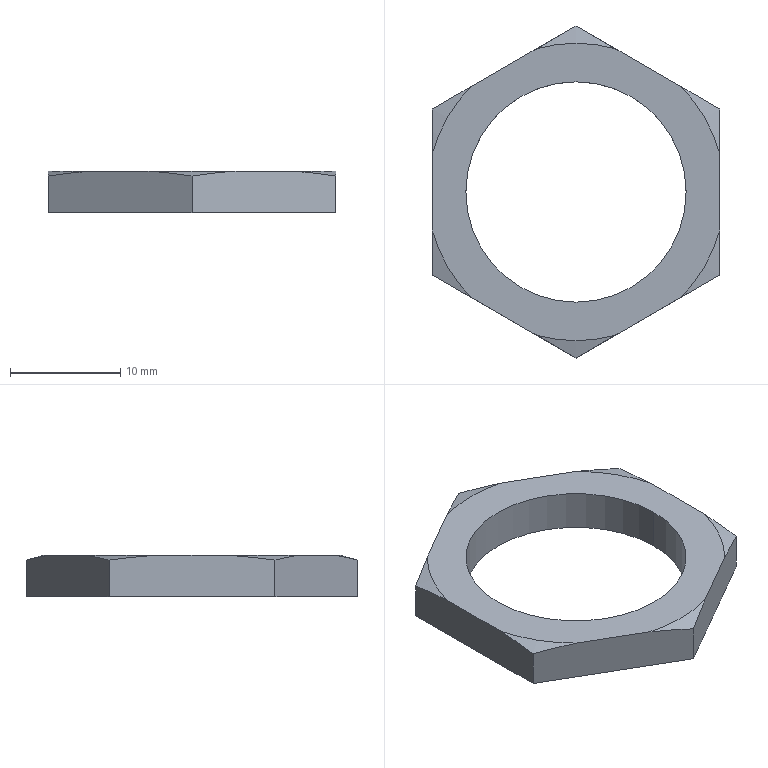Part | STEP file | GB/T 808 M20×1 | 1 solid | 16 faces | box 26.102 x 30.14 x 3.74 mm | volume 1028 mm3 | plane 8 | cone 6 | cylinder 2 | commonest cylinder face diameters 20 x2
STEP:
#1=CARTESIAN_POINT('',(-10.,0.,3.74));
#2=VERTEX_POINT('',#1);
#3=CARTESIAN_POINT('',(10.,0.,3.74));
#4=VERTEX_POINT('',#3);
#5=CARTESIAN_POINT('',(0.,0.,3.74));
#6=DIRECTION('',(0.,0.,1.));
#7=DIRECTION('',(1.,0.,0.));
#8=AXIS2_PLACEMENT_3D('',#5,#6,#7);
#9=CIRCLE('',#8,10.);
#10=EDGE_CURVE('',#2,#4,#9,.T.);
#11=ORIENTED_EDGE('',*,*,#10,.T.);
#12=CARTESIAN_POINT('',(10.,0.,0.));
#13=VERTEX_POINT('',#12);
#14=CARTESIAN_POINT('',(10.,0.,3.74));
#15=DIRECTION('',(0.,0.,-1.));
#16=VECTOR('',#15,1000.);
#17=LINE('',#14,#16);
#18=EDGE_CURVE('',#4,#13,#17,.T.);
#19=ORIENTED_EDGE('',*,*,#18,.T.);
#20=CARTESIAN_POINT('',(-10.,0.,0.));
#21=VERTEX_POINT('',#20);
#22=CARTESIAN_POINT('',(0.,0.,0.));
#23=DIRECTION('',(0.,0.,1.));
#24=DIRECTION('',(1.,0.,0.));
#25=AXIS2_PLACEMENT_3D('',#22,#23,#24);
#26=CIRCLE('',#25,10.);
#27=EDGE_CURVE('',#21,#13,#26,.T.);
#28=ORIENTED_EDGE('',*,*,#27,.F.);
#29=CARTESIAN_POINT('',(-10.,0.,3.74));
#30=DIRECTION('',(0.,0.,-1.));
#31=VECTOR('',#30,1000.);
#32=LINE('',#29,#31);
#33=EDGE_CURVE('',#2,#21,#32,.T.);
#34=ORIENTED_EDGE('',*,*,#33,.F.);
#35=EDGE_LOOP('',(#11,#19,#28,#34));
#36=FACE_OUTER_BOUND('',#35,.T.);
#37=CARTESIAN_POINT('',(0.,0.,3.74));
#38=DIRECTION('',(0.,0.,-1.));
#39=DIRECTION('',(-1.,0.,0.));
#40=AXIS2_PLACEMENT_3D('',#37,#38,#39);
#41=CYLINDRICAL_SURFACE('',#40,10.);
#42=ADVANCED_FACE('',(#36),#41,.F.);
#43=ORIENTED_EDGE('',*,*,#10,.F.);
#44=CARTESIAN_POINT('',(0.,0.,3.74));
#45=DIRECTION('',(0.,0.,1.));
#46=DIRECTION('',(1.,0.,0.));
#47=AXIS2_PLACEMENT_3D('',#44,#45,#46);
#48=CIRCLE('',#47,10.);
#49=EDGE_CURVE('',#4,#2,#48,.T.);
#50=ORIENTED_EDGE('',*,*,#49,.F.);
#51=EDGE_LOOP('',(#43,#50));
#52=FACE_BOUND('',#51,.T.);
#53=CARTESIAN_POINT('',(-9.516,9.576,3.74));
#54=VERTEX_POINT('',#53);
#55=CARTESIAN_POINT('',(-13.051,3.453,3.74));
#56=VERTEX_POINT('',#55);
#57=CARTESIAN_POINT('',(0.,0.,3.74));
#58=DIRECTION('',(0.,0.,1.));
#59=DIRECTION('',(1.,0.,0.));
#60=AXIS2_PLACEMENT_3D('',#57,#58,#59);
#61=CIRCLE('',#60,13.5);
#62=EDGE_CURVE('',#54,#56,#61,.T.);
#63=ORIENTED_EDGE('',*,*,#62,.T.);
#64=CARTESIAN_POINT('',(-13.051,-3.453,3.74));
#65=VERTEX_POINT('',#64);
#66=CARTESIAN_POINT('',(-13.051,7.535,3.74));
#67=DIRECTION('',(0.,-1.,0.));
#68=VECTOR('',#67,1000.);
#69=LINE('',#66,#68);
#70=EDGE_CURVE('',#56,#65,#69,.T.);
#71=ORIENTED_EDGE('',*,*,#70,.T.);
#72=CARTESIAN_POINT('',(-9.516,-9.576,3.74));
#73=VERTEX_POINT('',#72);
#74=CARTESIAN_POINT('',(0.,0.,3.74));
#75=DIRECTION('',(0.,0.,1.));
#76=DIRECTION('',(1.,0.,0.));
#77=AXIS2_PLACEMENT_3D('',#74,#75,#76);
#78=CIRCLE('',#77,13.5);
#79=EDGE_CURVE('',#65,#73,#78,.T.);
#80=ORIENTED_EDGE('',*,*,#79,.T.);
#81=CARTESIAN_POINT('',(-3.535,-13.029,3.74));
#82=VERTEX_POINT('',#81);
#83=CARTESIAN_POINT('',(-13.051,-7.535,3.74));
#84=DIRECTION('',(0.866,-0.5,0.));
#85=VECTOR('',#84,1000.);
#86=LINE('',#83,#85);
#87=EDGE_CURVE('',#73,#82,#86,.T.);
#88=ORIENTED_EDGE('',*,*,#87,.T.);
#89=CARTESIAN_POINT('',(3.535,-13.029,3.74));
#90=VERTEX_POINT('',#89);
#91=CARTESIAN_POINT('',(0.,0.,3.74));
#92=DIRECTION('',(0.,0.,1.));
#93=DIRECTION('',(1.,0.,0.));
#94=AXIS2_PLACEMENT_3D('',#91,#92,#93);
#95=CIRCLE('',#94,13.5);
#96=EDGE_CURVE('',#82,#90,#95,.T.);
#97=ORIENTED_EDGE('',*,*,#96,.T.);
#98=CARTESIAN_POINT('',(9.516,-9.576,3.74));
#99=VERTEX_POINT('',#98);
#100=CARTESIAN_POINT('',(0.,-15.07,3.74));
#101=DIRECTION('',(0.866,0.5,0.));
#102=VECTOR('',#101,1000.);
#103=LINE('',#100,#102);
#104=EDGE_CURVE('',#90,#99,#103,.T.);
#105=ORIENTED_EDGE('',*,*,#104,.T.);
#106=CARTESIAN_POINT('',(13.051,-3.453,3.74));
#107=VERTEX_POINT('',#106);
#108=CARTESIAN_POINT('',(0.,0.,3.74));
#109=DIRECTION('',(0.,0.,1.));
#110=DIRECTION('',(1.,0.,0.));
#111=AXIS2_PLACEMENT_3D('',#108,#109,#110);
#112=CIRCLE('',#111,13.5);
#113=EDGE_CURVE('',#99,#107,#112,.T.);
#114=ORIENTED_EDGE('',*,*,#113,.T.);
#115=CARTESIAN_POINT('',(13.051,3.453,3.74));
#116=VERTEX_POINT('',#115);
#117=CARTESIAN_POINT('',(13.051,-7.535,3.74));
#118=DIRECTION('',(0.,1.,0.));
#119=VECTOR('',#118,1000.);
#120=LINE('',#117,#119);
#121=EDGE_CURVE('',#107,#116,#120,.T.);
#122=ORIENTED_EDGE('',*,*,#121,.T.);
#123=CARTESIAN_POINT('',(9.516,9.576,3.74));
#124=VERTEX_POINT('',#123);
#125=CARTESIAN_POINT('',(0.,0.,3.74));
#126=DIRECTION('',(0.,0.,1.));
#127=DIRECTION('',(1.,0.,0.));
#128=AXIS2_PLACEMENT_3D('',#125,#126,#127);
#129=CIRCLE('',#128,13.5);
#130=EDGE_CURVE('',#116,#124,#129,.T.);
#131=ORIENTED_EDGE('',*,*,#130,.T.);
#132=CARTESIAN_POINT('',(3.535,13.029,3.74));
#133=VERTEX_POINT('',#132);
#134=CARTESIAN_POINT('',(13.051,7.535,3.74));
#135=DIRECTION('',(-0.866,0.5,0.));
#136=VECTOR('',#135,1000.);
#137=LINE('',#134,#136);
#138=EDGE_CURVE('',#124,#133,#137,.T.);
#139=ORIENTED_EDGE('',*,*,#138,.T.);
#140=CARTESIAN_POINT('',(-3.535,13.029,3.74));
#141=VERTEX_POINT('',#140);
#142=CARTESIAN_POINT('',(0.,0.,3.74));
#143=DIRECTION('',(0.,0.,1.));
#144=DIRECTION('',(1.,0.,0.));
#145=AXIS2_PLACEMENT_3D('',#142,#143,#144);
#146=CIRCLE('',#145,13.5);
#147=EDGE_CURVE('',#133,#141,#146,.T.);
#148=ORIENTED_EDGE('',*,*,#147,.T.);
#149=CARTESIAN_POINT('',(0.,15.07,3.74));
#150=DIRECTION('',(-0.866,-0.5,0.));
#151=VECTOR('',#150,1000.);
#152=LINE('',#149,#151);
#153=EDGE_CURVE('',#141,#54,#152,.T.);
#154=ORIENTED_EDGE('',*,*,#153,.T.);
#155=EDGE_LOOP('',(#63,#71,#80,#88,#97,#105,#114,#122,#131,#139,#148,#154));
#156=FACE_OUTER_BOUND('',#155,.T.);
#157=CARTESIAN_POINT('',(26.102,0.,3.74));
#158=DIRECTION('',(0.,0.,-1.));
#159=DIRECTION('',(-1.,0.,0.));
#160=AXIS2_PLACEMENT_3D('',#157,#158,#159);
#161=PLANE('',#160);
#162=ADVANCED_FACE('',(#52,#156),#161,.F.);
#163=CARTESIAN_POINT('',(13.051,7.535,3.319));
#164=VERTEX_POINT('',#163);
#165=CARTESIAN_POINT('',(13.051,7.535,3.319));
#166=CARTESIAN_POINT('',(11.876,8.213,3.501));
#167=CARTESIAN_POINT('',(10.698,8.893,3.646));
#168=CARTESIAN_POINT('',(9.516,9.576,3.74));
#169=B_SPLINE_CURVE_WITH_KNOTS('',3,(#165,#166,#167,#168),.UNSPECIFIED.,.F.,.F.,(4,4),(0.0109,0.01501),.UNSPECIFIED.);
#170=EDGE_CURVE('',#164,#124,#169,.T.);
#171=ORIENTED_EDGE('',*,*,#170,.F.);
#172=CARTESIAN_POINT('',(13.051,7.535,0.));
#173=VERTEX_POINT('',#172);
#174=CARTESIAN_POINT('',(13.051,7.535,3.74));
#175=DIRECTION('',(0.,0.,-1.));
#176=VECTOR('',#175,1000.);
#177=LINE('',#174,#176);
#178=EDGE_CURVE('',#164,#173,#177,.T.);
#179=ORIENTED_EDGE('',*,*,#178,.T.);
#180=CARTESIAN_POINT('',(0.,15.07,0.));
#181=VERTEX_POINT('',#180);
#182=CARTESIAN_POINT('',(13.051,7.535,0.));
#183=DIRECTION('',(-0.866,0.5,0.));
#184=VECTOR('',#183,1000.);
#185=LINE('',#182,#184);
#186=EDGE_CURVE('',#173,#181,#185,.T.);
#187=ORIENTED_EDGE('',*,*,#186,.T.);
#188=CARTESIAN_POINT('',(0.,15.07,3.319));
#189=VERTEX_POINT('',#188);
#190=CARTESIAN_POINT('',(0.,15.07,3.74));
#191=DIRECTION('',(0.,0.,-1.));
#192=VECTOR('',#191,1000.);
#193=LINE('',#190,#192);
#194=EDGE_CURVE('',#189,#181,#193,.T.);
#195=ORIENTED_EDGE('',*,*,#194,.F.);
#196=CARTESIAN_POINT('',(3.535,13.029,3.74));
#197=CARTESIAN_POINT('',(2.946,13.369,3.693));
#198=CARTESIAN_POINT('',(2.354,13.711,3.634));
#199=CARTESIAN_POINT('',(1.175,14.392,3.492));
#200=CARTESIAN_POINT('',(0.5867,14.731,3.41));
#201=CARTESIAN_POINT('',(0.,15.07,3.319));
#202=B_SPLINE_CURVE_WITH_KNOTS('',3,(#196,#197,#198,#199,#200,#201),.UNSPECIFIED.,.F.,.F.,(4,2,4),(0.02188,0.0239,0.02591),.UNSPECIFIED.);
#203=EDGE_CURVE('',#133,#189,#202,.T.);
#204=ORIENTED_EDGE('',*,*,#203,.F.);
#205=ORIENTED_EDGE('',*,*,#138,.F.);
#206=EDGE_LOOP('',(#171,#179,#187,#195,#204,#205));
#207=FACE_OUTER_BOUND('',#206,.T.);
#208=CARTESIAN_POINT('',(13.051,7.535,3.74));
#209=DIRECTION('',(-0.5,-0.866,0.));
#210=DIRECTION('',(0.866,-0.5,0.));
#211=AXIS2_PLACEMENT_3D('',#208,#209,#210);
#212=PLANE('',#211);
#213=ADVANCED_FACE('',(#207),#212,.F.);
#214=CARTESIAN_POINT('',(0.,15.07,3.319));
#215=CARTESIAN_POINT('',(-1.175,14.392,3.501));
#216=CARTESIAN_POINT('',(-2.353,13.712,3.646));
#217=CARTESIAN_POINT('',(-3.535,13.029,3.74));
#218=B_SPLINE_CURVE_WITH_KNOTS('',3,(#214,#215,#216,#217),.UNSPECIFIED.,.F.,.F.,(4,4),(0.0109,0.01501),.UNSPECIFIED.);
#219=EDGE_CURVE('',#189,#141,#218,.T.);
#220=ORIENTED_EDGE('',*,*,#219,.F.);
#221=ORIENTED_EDGE('',*,*,#194,.T.);
#222=CARTESIAN_POINT('',(-13.051,7.535,0.));
#223=VERTEX_POINT('',#222);
#224=CARTESIAN_POINT('',(0.,15.07,0.));
#225=DIRECTION('',(-0.866,-0.5,0.));
#226=VECTOR('',#225,1000.);
#227=LINE('',#224,#226);
#228=EDGE_CURVE('',#181,#223,#227,.T.);
#229=ORIENTED_EDGE('',*,*,#228,.T.);
#230=CARTESIAN_POINT('',(-13.051,7.535,3.319));
#231=VERTEX_POINT('',#230);
#232=CARTESIAN_POINT('',(-13.051,7.535,3.74));
#233=DIRECTION('',(0.,0.,-1.));
#234=VECTOR('',#233,1000.);
#235=LINE('',#232,#234);
#236=EDGE_CURVE('',#231,#223,#235,.T.);
#237=ORIENTED_EDGE('',*,*,#236,.F.);
#238=CARTESIAN_POINT('',(-9.516,9.576,3.74));
#239=CARTESIAN_POINT('',(-10.105,9.236,3.693));
#240=CARTESIAN_POINT('',(-10.697,8.894,3.634));
#241=CARTESIAN_POINT('',(-11.876,8.213,3.492));
#242=CARTESIAN_POINT('',(-12.464,7.874,3.41));
#243=CARTESIAN_POINT('',(-13.051,7.535,3.319));
#244=B_SPLINE_CURVE_WITH_KNOTS('',3,(#238,#239,#240,#241,#242,#243),.UNSPECIFIED.,.F.,.F.,(4,2,4),(0.02188,0.0239,0.02591),.UNSPECIFIED.);
#245=EDGE_CURVE('',#54,#231,#244,.T.);
#246=ORIENTED_EDGE('',*,*,#245,.F.);
#247=ORIENTED_EDGE('',*,*,#153,.F.);
#248=EDGE_LOOP('',(#220,#221,#229,#237,#246,#247));
#249=FACE_OUTER_BOUND('',#248,.T.);
#250=CARTESIAN_POINT('',(0.,15.07,3.74));
#251=DIRECTION('',(0.5,-0.866,0.));
#252=DIRECTION('',(0.866,0.5,0.));
#253=AXIS2_PLACEMENT_3D('',#250,#251,#252);
#254=PLANE('',#253);
#255=ADVANCED_FACE('',(#249),#254,.F.);
#256=CARTESIAN_POINT('',(-13.051,7.535,3.319));
#257=CARTESIAN_POINT('',(-13.051,6.178,3.501));
#258=CARTESIAN_POINT('',(-13.051,4.818,3.646));
#259=CARTESIAN_POINT('',(-13.051,3.453,3.74));
#260=B_SPLINE_CURVE_WITH_KNOTS('',3,(#256,#257,#258,#259),.UNSPECIFIED.,.F.,.F.,(4,4),(0.00943,0.01353),.UNSPECIFIED.);
#261=EDGE_CURVE('',#231,#56,#260,.T.);
#262=ORIENTED_EDGE('',*,*,#261,.F.);
#263=ORIENTED_EDGE('',*,*,#236,.T.);
#264=CARTESIAN_POINT('',(-13.051,-7.535,0.));
#265=VERTEX_POINT('',#264);
#266=CARTESIAN_POINT('',(-13.051,7.535,0.));
#267=DIRECTION('',(0.,-1.,0.));
#268=VECTOR('',#267,1000.);
#269=LINE('',#266,#268);
#270=EDGE_CURVE('',#223,#265,#269,.T.);
#271=ORIENTED_EDGE('',*,*,#270,.T.);
#272=CARTESIAN_POINT('',(-13.051,-7.535,3.319));
#273=VERTEX_POINT('',#272);
#274=CARTESIAN_POINT('',(-13.051,-7.535,3.74));
#275=DIRECTION('',(0.,0.,-1.));
#276=VECTOR('',#275,1000.);
#277=LINE('',#274,#276);
#278=EDGE_CURVE('',#273,#265,#277,.T.);
#279=ORIENTED_EDGE('',*,*,#278,.F.);
#280=CARTESIAN_POINT('',(-13.051,-3.453,3.74));
#281=CARTESIAN_POINT('',(-13.051,-4.133,3.693));
#282=CARTESIAN_POINT('',(-13.051,-4.816,3.634));
#283=CARTESIAN_POINT('',(-13.051,-6.178,3.492));
#284=CARTESIAN_POINT('',(-13.051,-6.857,3.41));
#285=CARTESIAN_POINT('',(-13.051,-7.535,3.319));
#286=B_SPLINE_CURVE_WITH_KNOTS('',3,(#280,#281,#282,#283,#284,#285),.UNSPECIFIED.,.F.,.F.,(4,2,4),(0.02041,0.02243,0.02445),.UNSPECIFIED.);
#287=EDGE_CURVE('',#65,#273,#286,.T.);
#288=ORIENTED_EDGE('',*,*,#287,.F.);
#289=ORIENTED_EDGE('',*,*,#70,.F.);
#290=EDGE_LOOP('',(#262,#263,#271,#279,#288,#289));
#291=FACE_OUTER_BOUND('',#290,.T.);
#292=CARTESIAN_POINT('',(-13.051,7.535,3.74));
#293=DIRECTION('',(1.,0.,0.));
#294=DIRECTION('',(0.,1.,0.));
#295=AXIS2_PLACEMENT_3D('',#292,#293,#294);
#296=PLANE('',#295);
#297=ADVANCED_FACE('',(#291),#296,.F.);
#298=CARTESIAN_POINT('',(-13.051,-7.535,3.319));
#299=CARTESIAN_POINT('',(-11.876,-8.213,3.501));
#300=CARTESIAN_POINT('',(-10.698,-8.893,3.646));
#301=CARTESIAN_POINT('',(-9.516,-9.576,3.74));
#302=B_SPLINE_CURVE_WITH_KNOTS('',3,(#298,#299,#300,#301),.UNSPECIFIED.,.F.,.F.,(4,4),(0.0109,0.01501),.UNSPECIFIED.);
#303=EDGE_CURVE('',#273,#73,#302,.T.);
#304=ORIENTED_EDGE('',*,*,#303,.F.);
#305=ORIENTED_EDGE('',*,*,#278,.T.);
#306=CARTESIAN_POINT('',(0.,-15.07,0.));
#307=VERTEX_POINT('',#306);
#308=CARTESIAN_POINT('',(-13.051,-7.535,0.));
#309=DIRECTION('',(0.866,-0.5,0.));
#310=VECTOR('',#309,1000.);
#311=LINE('',#308,#310);
#312=EDGE_CURVE('',#265,#307,#311,.T.);
#313=ORIENTED_EDGE('',*,*,#312,.T.);
#314=CARTESIAN_POINT('',(0.,-15.07,3.319));
#315=VERTEX_POINT('',#314);
#316=CARTESIAN_POINT('',(0.,-15.07,3.74));
#317=DIRECTION('',(0.,0.,-1.));
#318=VECTOR('',#317,1000.);
#319=LINE('',#316,#318);
#320=EDGE_CURVE('',#315,#307,#319,.T.);
#321=ORIENTED_EDGE('',*,*,#320,.F.);
#322=CARTESIAN_POINT('',(-3.535,-13.029,3.74));
#323=CARTESIAN_POINT('',(-2.946,-13.369,3.693));
#324=CARTESIAN_POINT('',(-2.354,-13.711,3.634));
#325=CARTESIAN_POINT('',(-1.175,-14.392,3.492));
#326=CARTESIAN_POINT('',(-0.5867,-14.731,3.41));
#327=CARTESIAN_POINT('',(0.,-15.07,3.319));
#328=B_SPLINE_CURVE_WITH_KNOTS('',3,(#322,#323,#324,#325,#326,#327),.UNSPECIFIED.,.F.,.F.,(4,2,4),(0.02188,0.0239,0.02591),.UNSPECIFIED.);
#329=EDGE_CURVE('',#82,#315,#328,.T.);
#330=ORIENTED_EDGE('',*,*,#329,.F.);
#331=ORIENTED_EDGE('',*,*,#87,.F.);
#332=EDGE_LOOP('',(#304,#305,#313,#321,#330,#331));
#333=FACE_OUTER_BOUND('',#332,.T.);
#334=CARTESIAN_POINT('',(-13.051,-7.535,3.74));
#335=DIRECTION('',(0.5,0.866,0.));
#336=DIRECTION('',(-0.866,0.5,0.));
#337=AXIS2_PLACEMENT_3D('',#334,#335,#336);
#338=PLANE('',#337);
#339=ADVANCED_FACE('',(#333),#338,.F.);
#340=CARTESIAN_POINT('',(0.,-15.07,3.319));
#341=CARTESIAN_POINT('',(1.175,-14.392,3.501));
#342=CARTESIAN_POINT('',(2.353,-13.712,3.646));
#343=CARTESIAN_POINT('',(3.535,-13.029,3.74));
#344=B_SPLINE_CURVE_WITH_KNOTS('',3,(#340,#341,#342,#343),.UNSPECIFIED.,.F.,.F.,(4,4),(0.0109,0.01501),.UNSPECIFIED.);
#345=EDGE_CURVE('',#315,#90,#344,.T.);
#346=ORIENTED_EDGE('',*,*,#345,.F.);
#347=ORIENTED_EDGE('',*,*,#320,.T.);
#348=CARTESIAN_POINT('',(13.051,-7.535,0.));
#349=VERTEX_POINT('',#348);
#350=CARTESIAN_POINT('',(0.,-15.07,0.));
#351=DIRECTION('',(0.866,0.5,0.));
#352=VECTOR('',#351,1000.);
#353=LINE('',#350,#352);
#354=EDGE_CURVE('',#307,#349,#353,.T.);
#355=ORIENTED_EDGE('',*,*,#354,.T.);
#356=CARTESIAN_POINT('',(13.051,-7.535,3.319));
#357=VERTEX_POINT('',#356);
#358=CARTESIAN_POINT('',(13.051,-7.535,3.74));
#359=DIRECTION('',(0.,0.,-1.));
#360=VECTOR('',#359,1000.);
#361=LINE('',#358,#360);
#362=EDGE_CURVE('',#357,#349,#361,.T.);
#363=ORIENTED_EDGE('',*,*,#362,.F.);
#364=CARTESIAN_POINT('',(9.516,-9.576,3.74));
#365=CARTESIAN_POINT('',(10.105,-9.236,3.693));
#366=CARTESIAN_POINT('',(10.697,-8.894,3.634));
#367=CARTESIAN_POINT('',(11.876,-8.213,3.492));
#368=CARTESIAN_POINT('',(12.464,-7.874,3.41));
#369=CARTESIAN_POINT('',(13.051,-7.535,3.319));
#370=B_SPLINE_CURVE_WITH_KNOTS('',3,(#364,#365,#366,#367,#368,#369),.UNSPECIFIED.,.F.,.F.,(4,2,4),(0.02188,0.0239,0.02591),.UNSPECIFIED.);
#371=EDGE_CURVE('',#99,#357,#370,.T.);
#372=ORIENTED_EDGE('',*,*,#371,.F.);
#373=ORIENTED_EDGE('',*,*,#104,.F.);
#374=EDGE_LOOP('',(#346,#347,#355,#363,#372,#373));
#375=FACE_OUTER_BOUND('',#374,.T.);
#376=CARTESIAN_POINT('',(0.,-15.07,3.74));
#377=DIRECTION('',(-0.5,0.866,0.));
#378=DIRECTION('',(-0.866,-0.5,0.));
#379=AXIS2_PLACEMENT_3D('',#376,#377,#378);
#380=PLANE('',#379);
#381=ADVANCED_FACE('',(#375),#380,.F.);
#382=CARTESIAN_POINT('',(13.051,-7.535,3.319));
#383=CARTESIAN_POINT('',(13.051,-6.178,3.501));
#384=CARTESIAN_POINT('',(13.051,-4.818,3.646));
#385=CARTESIAN_POINT('',(13.051,-3.453,3.74));
#386=B_SPLINE_CURVE_WITH_KNOTS('',3,(#382,#383,#384,#385),.UNSPECIFIED.,.F.,.F.,(4,4),(0.00943,0.01353),.UNSPECIFIED.);
#387=EDGE_CURVE('',#357,#107,#386,.T.);
#388=ORIENTED_EDGE('',*,*,#387,.F.);
#389=ORIENTED_EDGE('',*,*,#362,.T.);
#390=CARTESIAN_POINT('',(13.051,-7.535,0.));
#391=DIRECTION('',(0.,1.,0.));
#392=VECTOR('',#391,1000.);
#393=LINE('',#390,#392);
#394=EDGE_CURVE('',#349,#173,#393,.T.);
#395=ORIENTED_EDGE('',*,*,#394,.T.);
#396=ORIENTED_EDGE('',*,*,#178,.F.);
#397=CARTESIAN_POINT('',(13.051,3.453,3.74));
#398=CARTESIAN_POINT('',(13.051,4.133,3.693));
#399=CARTESIAN_POINT('',(13.051,4.816,3.634));
#400=CARTESIAN_POINT('',(13.051,6.178,3.492));
#401=CARTESIAN_POINT('',(13.051,6.857,3.41));
#402=CARTESIAN_POINT('',(13.051,7.535,3.319));
#403=B_SPLINE_CURVE_WITH_KNOTS('',3,(#397,#398,#399,#400,#401,#402),.UNSPECIFIED.,.F.,.F.,(4,2,4),(0.02041,0.02243,0.02445),.UNSPECIFIED.);
#404=EDGE_CURVE('',#116,#164,#403,.T.);
#405=ORIENTED_EDGE('',*,*,#404,.F.);
#406=ORIENTED_EDGE('',*,*,#121,.F.);
#407=EDGE_LOOP('',(#388,#389,#395,#396,#405,#406));
#408=FACE_OUTER_BOUND('',#407,.T.);
#409=CARTESIAN_POINT('',(13.051,-7.535,3.74));
#410=DIRECTION('',(-1.,0.,0.));
#411=DIRECTION('',(0.,-1.,0.));
#412=AXIS2_PLACEMENT_3D('',#409,#410,#411);
#413=PLANE('',#412);
#414=ADVANCED_FACE('',(#408),#413,.F.);
#415=ORIENTED_EDGE('',*,*,#186,.F.);
#416=ORIENTED_EDGE('',*,*,#394,.F.);
#417=ORIENTED_EDGE('',*,*,#354,.F.);
#418=ORIENTED_EDGE('',*,*,#312,.F.);
#419=ORIENTED_EDGE('',*,*,#270,.F.);
#420=ORIENTED_EDGE('',*,*,#228,.F.);
#421=EDGE_LOOP('',(#415,#416,#417,#418,#419,#420));
#422=FACE_OUTER_BOUND('',#421,.T.);
#423=ORIENTED_EDGE('',*,*,#27,.T.);
#424=CARTESIAN_POINT('',(0.,0.,0.));
#425=DIRECTION('',(0.,0.,1.));
#426=DIRECTION('',(1.,0.,0.));
#427=AXIS2_PLACEMENT_3D('',#424,#425,#426);
#428=CIRCLE('',#427,10.);
#429=EDGE_CURVE('',#13,#21,#428,.T.);
#430=ORIENTED_EDGE('',*,*,#429,.T.);
#431=EDGE_LOOP('',(#423,#430));
#432=FACE_BOUND('',#431,.T.);
#433=CARTESIAN_POINT('',(26.102,0.,0.));
#434=DIRECTION('',(0.,0.,-1.));
#435=DIRECTION('',(-1.,0.,0.));
#436=AXIS2_PLACEMENT_3D('',#433,#434,#435);
#437=PLANE('',#436);
#438=ADVANCED_FACE('',(#422,#432),#437,.T.);
#439=ORIENTED_EDGE('',*,*,#18,.F.);
#440=ORIENTED_EDGE('',*,*,#49,.T.);
#441=ORIENTED_EDGE('',*,*,#33,.T.);
#442=ORIENTED_EDGE('',*,*,#429,.F.);
#443=EDGE_LOOP('',(#439,#440,#441,#442));
#444=FACE_OUTER_BOUND('',#443,.T.);
#445=CARTESIAN_POINT('',(0.,0.,3.74));
#446=DIRECTION('',(0.,0.,-1.));
#447=DIRECTION('',(-1.,0.,0.));
#448=AXIS2_PLACEMENT_3D('',#445,#446,#447);
#449=CYLINDRICAL_SURFACE('',#448,10.);
#450=ADVANCED_FACE('',(#444),#449,.F.);
#451=ORIENTED_EDGE('',*,*,#170,.T.);
#452=ORIENTED_EDGE('',*,*,#130,.F.);
#453=ORIENTED_EDGE('',*,*,#404,.T.);
#454=EDGE_LOOP('',(#451,#452,#453));
#455=FACE_OUTER_BOUND('',#454,.T.);
#456=CARTESIAN_POINT('',(0.,0.,3.74));
#457=DIRECTION('',(0.,0.,-1.));
#458=DIRECTION('',(1.,0.,0.));
#459=AXIS2_PLACEMENT_3D('',#456,#457,#458);
#460=CONICAL_SURFACE('',#459,13.5,1.309);
#461=ADVANCED_FACE('',(#455),#460,.T.);
#462=ORIENTED_EDGE('',*,*,#371,.T.);
#463=ORIENTED_EDGE('',*,*,#387,.T.);
#464=ORIENTED_EDGE('',*,*,#113,.F.);
#465=EDGE_LOOP('',(#462,#463,#464));
#466=FACE_OUTER_BOUND('',#465,.T.);
#467=CARTESIAN_POINT('',(0.,0.,3.74));
#468=DIRECTION('',(0.,0.,-1.));
#469=DIRECTION('',(1.,0.,0.));
#470=AXIS2_PLACEMENT_3D('',#467,#468,#469);
#471=CONICAL_SURFACE('',#470,13.5,1.309);
#472=ADVANCED_FACE('',(#466),#471,.T.);
#473=ORIENTED_EDGE('',*,*,#329,.T.);
#474=ORIENTED_EDGE('',*,*,#345,.T.);
#475=ORIENTED_EDGE('',*,*,#96,.F.);
#476=EDGE_LOOP('',(#473,#474,#475));
#477=FACE_OUTER_BOUND('',#476,.T.);
#478=CARTESIAN_POINT('',(0.,0.,3.74));
#479=DIRECTION('',(0.,0.,-1.));
#480=DIRECTION('',(1.,0.,0.));
#481=AXIS2_PLACEMENT_3D('',#478,#479,#480);
#482=CONICAL_SURFACE('',#481,13.5,1.309);
#483=ADVANCED_FACE('',(#477),#482,.T.);
#484=ORIENTED_EDGE('',*,*,#287,.T.);
#485=ORIENTED_EDGE('',*,*,#303,.T.);
#486=ORIENTED_EDGE('',*,*,#79,.F.);
#487=EDGE_LOOP('',(#484,#485,#486));
#488=FACE_OUTER_BOUND('',#487,.T.);
#489=CARTESIAN_POINT('',(0.,0.,3.74));
#490=DIRECTION('',(0.,0.,-1.));
#491=DIRECTION('',(1.,0.,0.));
#492=AXIS2_PLACEMENT_3D('',#489,#490,#491);
#493=CONICAL_SURFACE('',#492,13.5,1.309);
#494=ADVANCED_FACE('',(#488),#493,.T.);
#495=ORIENTED_EDGE('',*,*,#245,.T.);
#496=ORIENTED_EDGE('',*,*,#261,.T.);
#497=ORIENTED_EDGE('',*,*,#62,.F.);
#498=EDGE_LOOP('',(#495,#496,#497));
#499=FACE_OUTER_BOUND('',#498,.T.);
#500=CARTESIAN_POINT('',(0.,0.,3.74));
#501=DIRECTION('',(0.,0.,-1.));
#502=DIRECTION('',(1.,0.,0.));
#503=AXIS2_PLACEMENT_3D('',#500,#501,#502);
#504=CONICAL_SURFACE('',#503,13.5,1.309);
#505=ADVANCED_FACE('',(#499),#504,.T.);
#506=ORIENTED_EDGE('',*,*,#203,.T.);
#507=ORIENTED_EDGE('',*,*,#219,.T.);
#508=ORIENTED_EDGE('',*,*,#147,.F.);
#509=EDGE_LOOP('',(#506,#507,#508));
#510=FACE_OUTER_BOUND('',#509,.T.);
#511=CARTESIAN_POINT('',(0.,0.,3.74));
#512=DIRECTION('',(0.,0.,-1.));
#513=DIRECTION('',(1.,0.,0.));
#514=AXIS2_PLACEMENT_3D('',#511,#512,#513);
#515=CONICAL_SURFACE('',#514,13.5,1.309);
#516=ADVANCED_FACE('',(#510),#515,.T.);
#517=CLOSED_SHELL('',(#42,#162,#213,#255,#297,#339,#381,#414,#438,#450,#461,#472,#483,#494,#505,#516));
#518=MANIFOLD_SOLID_BREP('',#517);
#519=CARTESIAN_POINT('',(0.,0.,0.));
#520=DIRECTION('',(0.,0.,1.));
#521=DIRECTION('',(1.,0.,0.));
#522=AXIS2_PLACEMENT_3D('',#519,#520,#521);
#523=(LENGTH_UNIT()NAMED_UNIT(*)SI_UNIT(.MILLI.,.METRE.));
#524=UNCERTAINTY_MEASURE_WITH_UNIT(LENGTH_MEASURE(0.00001),#523,'','');
#525=(NAMED_UNIT(*)PLANE_ANGLE_UNIT()SI_UNIT($,.RADIAN.));
#526=(NAMED_UNIT(*)SI_UNIT($,.STERADIAN.)SOLID_ANGLE_UNIT());
#527=(GEOMETRIC_REPRESENTATION_CONTEXT(3)GLOBAL_UNCERTAINTY_ASSIGNED_CONTEXT((#524))GLOBAL_UNIT_ASSIGNED_CONTEXT((#523,#525,#526))REPRESENTATION_CONTEXT('',''));
#528=ADVANCED_BREP_SHAPE_REPRESENTATION('',(#518,#522),#527);